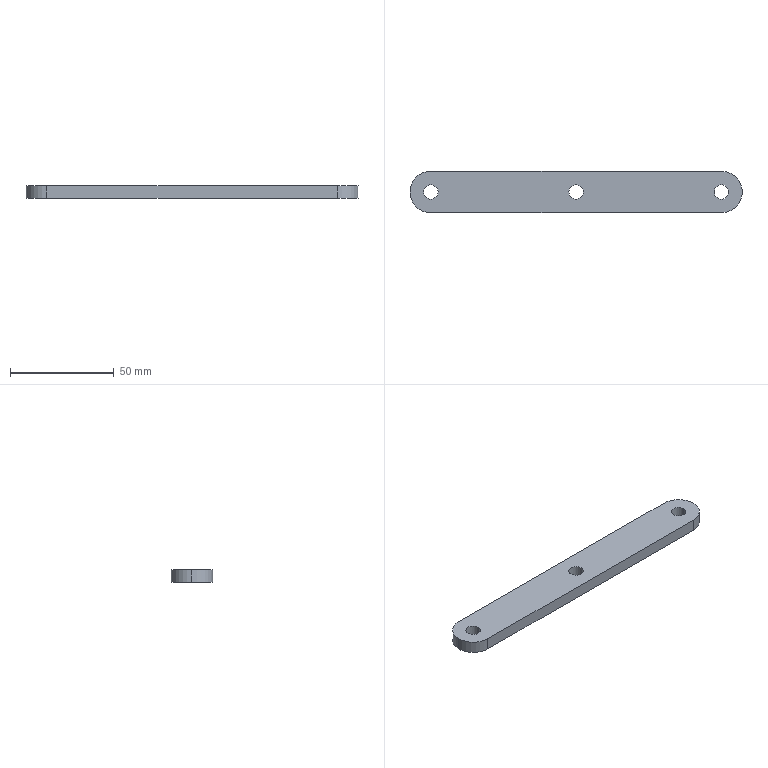Part | SolidWorks | features ICE 2, Extrusion 1 | 1 solid | 13 faces | box 160 x 20 x 6 mm | volume 17992 mm3 | cylinder 9 | plane 4 | commonest cylinder face diameters 7 x6 20 x3
STEP:
#1=CARTESIAN_POINT('',(66.5,0.,0.));
#2=VERTEX_POINT('',#1);
#3=CARTESIAN_POINT('',(73.5,0.,0.));
#4=VERTEX_POINT('',#3);
#5=CARTESIAN_POINT('',(70.,0.,0.));
#6=DIRECTION('',(0.,0.,1.));
#7=DIRECTION('',(1.,0.,0.));
#8=AXIS2_PLACEMENT_3D('',#5,#6,#7);
#9=CIRCLE('',#8,3.5);
#10=EDGE_CURVE('',#2,#4,#9,.T.);
#11=ORIENTED_EDGE('',*,*,#10,.F.);
#12=CARTESIAN_POINT('',(66.5,0.,6.));
#13=VERTEX_POINT('',#12);
#14=CARTESIAN_POINT('',(66.5,0.,-4.));
#15=DIRECTION('',(0.,0.,1.));
#16=VECTOR('',#15,1000.);
#17=LINE('',#14,#16);
#18=EDGE_CURVE('',#2,#13,#17,.T.);
#19=ORIENTED_EDGE('',*,*,#18,.T.);
#20=CARTESIAN_POINT('',(73.5,0.,6.));
#21=VERTEX_POINT('',#20);
#22=CARTESIAN_POINT('',(70.,0.,6.));
#23=DIRECTION('',(0.,0.,1.));
#24=DIRECTION('',(1.,0.,0.));
#25=AXIS2_PLACEMENT_3D('',#22,#23,#24);
#26=CIRCLE('',#25,3.5);
#27=EDGE_CURVE('',#13,#21,#26,.T.);
#28=ORIENTED_EDGE('',*,*,#27,.T.);
#29=CARTESIAN_POINT('',(73.5,0.,-4.));
#30=DIRECTION('',(0.,0.,1.));
#31=VECTOR('',#30,1000.);
#32=LINE('',#29,#31);
#33=EDGE_CURVE('',#4,#21,#32,.T.);
#34=ORIENTED_EDGE('',*,*,#33,.F.);
#35=EDGE_LOOP('',(#11,#19,#28,#34));
#36=FACE_OUTER_BOUND('',#35,.T.);
#37=CARTESIAN_POINT('',(70.,0.,-4.));
#38=DIRECTION('',(0.,0.,1.));
#39=DIRECTION('',(1.,0.,0.));
#40=AXIS2_PLACEMENT_3D('',#37,#38,#39);
#41=CYLINDRICAL_SURFACE('',#40,3.5);
#42=ADVANCED_FACE('',(#36),#41,.F.);
#43=CARTESIAN_POINT('',(136.5,0.,0.));
#44=VERTEX_POINT('',#43);
#45=CARTESIAN_POINT('',(143.5,0.,0.));
#46=VERTEX_POINT('',#45);
#47=CARTESIAN_POINT('',(140.,0.,0.));
#48=DIRECTION('',(0.,0.,1.));
#49=DIRECTION('',(1.,0.,0.));
#50=AXIS2_PLACEMENT_3D('',#47,#48,#49);
#51=CIRCLE('',#50,3.5);
#52=EDGE_CURVE('',#44,#46,#51,.T.);
#53=ORIENTED_EDGE('',*,*,#52,.F.);
#54=CARTESIAN_POINT('',(136.5,0.,6.));
#55=VERTEX_POINT('',#54);
#56=CARTESIAN_POINT('',(136.5,0.,-89.));
#57=DIRECTION('',(0.,0.,1.));
#58=VECTOR('',#57,1000.);
#59=LINE('',#56,#58);
#60=EDGE_CURVE('',#44,#55,#59,.T.);
#61=ORIENTED_EDGE('',*,*,#60,.T.);
#62=CARTESIAN_POINT('',(143.5,0.,6.));
#63=VERTEX_POINT('',#62);
#64=CARTESIAN_POINT('',(140.,0.,6.));
#65=DIRECTION('',(0.,0.,1.));
#66=DIRECTION('',(1.,0.,0.));
#67=AXIS2_PLACEMENT_3D('',#64,#65,#66);
#68=CIRCLE('',#67,3.5);
#69=EDGE_CURVE('',#55,#63,#68,.T.);
#70=ORIENTED_EDGE('',*,*,#69,.T.);
#71=CARTESIAN_POINT('',(143.5,0.,-89.));
#72=DIRECTION('',(0.,0.,1.));
#73=VECTOR('',#72,1000.);
#74=LINE('',#71,#73);
#75=EDGE_CURVE('',#46,#63,#74,.T.);
#76=ORIENTED_EDGE('',*,*,#75,.F.);
#77=EDGE_LOOP('',(#53,#61,#70,#76));
#78=FACE_OUTER_BOUND('',#77,.T.);
#79=CARTESIAN_POINT('',(140.,0.,-89.));
#80=DIRECTION('',(0.,0.,1.));
#81=DIRECTION('',(1.,0.,0.));
#82=AXIS2_PLACEMENT_3D('',#79,#80,#81);
#83=CYLINDRICAL_SURFACE('',#82,3.5);
#84=ADVANCED_FACE('',(#78),#83,.F.);
#85=CARTESIAN_POINT('',(-3.5,0.,0.));
#86=VERTEX_POINT('',#85);
#87=CARTESIAN_POINT('',(3.5,0.,0.));
#88=VERTEX_POINT('',#87);
#89=CARTESIAN_POINT('',(0.,0.,0.));
#90=DIRECTION('',(0.,0.,1.));
#91=DIRECTION('',(1.,0.,0.));
#92=AXIS2_PLACEMENT_3D('',#89,#90,#91);
#93=CIRCLE('',#92,3.5);
#94=EDGE_CURVE('',#86,#88,#93,.T.);
#95=ORIENTED_EDGE('',*,*,#94,.F.);
#96=CARTESIAN_POINT('',(-3.5,0.,6.));
#97=VERTEX_POINT('',#96);
#98=CARTESIAN_POINT('',(-3.5,0.,-89.));
#99=DIRECTION('',(0.,0.,1.));
#100=VECTOR('',#99,1000.);
#101=LINE('',#98,#100);
#102=EDGE_CURVE('',#86,#97,#101,.T.);
#103=ORIENTED_EDGE('',*,*,#102,.T.);
#104=CARTESIAN_POINT('',(3.5,0.,6.));
#105=VERTEX_POINT('',#104);
#106=CARTESIAN_POINT('',(0.,0.,6.));
#107=DIRECTION('',(0.,0.,1.));
#108=DIRECTION('',(1.,0.,0.));
#109=AXIS2_PLACEMENT_3D('',#106,#107,#108);
#110=CIRCLE('',#109,3.5);
#111=EDGE_CURVE('',#97,#105,#110,.T.);
#112=ORIENTED_EDGE('',*,*,#111,.T.);
#113=CARTESIAN_POINT('',(3.5,0.,-89.));
#114=DIRECTION('',(0.,0.,1.));
#115=VECTOR('',#114,1000.);
#116=LINE('',#113,#115);
#117=EDGE_CURVE('',#88,#105,#116,.T.);
#118=ORIENTED_EDGE('',*,*,#117,.F.);
#119=EDGE_LOOP('',(#95,#103,#112,#118));
#120=FACE_OUTER_BOUND('',#119,.T.);
#121=CARTESIAN_POINT('',(0.,0.,-89.));
#122=DIRECTION('',(0.,0.,1.));
#123=DIRECTION('',(1.,0.,0.));
#124=AXIS2_PLACEMENT_3D('',#121,#122,#123);
#125=CYLINDRICAL_SURFACE('',#124,3.5);
#126=ADVANCED_FACE('',(#120),#125,.F.);
#127=CARTESIAN_POINT('',(-10.,0.,6.));
#128=VERTEX_POINT('',#127);
#129=CARTESIAN_POINT('',(0.,-10.,6.));
#130=VERTEX_POINT('',#129);
#131=CARTESIAN_POINT('',(0.,0.,6.));
#132=DIRECTION('',(0.,0.,1.));
#133=DIRECTION('',(1.,0.,0.));
#134=AXIS2_PLACEMENT_3D('',#131,#132,#133);
#135=CIRCLE('',#134,10.);
#136=EDGE_CURVE('',#128,#130,#135,.T.);
#137=ORIENTED_EDGE('',*,*,#136,.F.);
#138=CARTESIAN_POINT('',(-10.,0.,0.));
#139=VERTEX_POINT('',#138);
#140=CARTESIAN_POINT('',(-10.,0.,6.));
#141=DIRECTION('',(0.,0.,-1.));
#142=VECTOR('',#141,1000.);
#143=LINE('',#140,#142);
#144=EDGE_CURVE('',#128,#139,#143,.T.);
#145=ORIENTED_EDGE('',*,*,#144,.T.);
#146=CARTESIAN_POINT('',(0.,-10.,0.));
#147=VERTEX_POINT('',#146);
#148=CARTESIAN_POINT('',(0.,0.,0.));
#149=DIRECTION('',(0.,0.,1.));
#150=DIRECTION('',(1.,0.,0.));
#151=AXIS2_PLACEMENT_3D('',#148,#149,#150);
#152=CIRCLE('',#151,10.);
#153=EDGE_CURVE('',#139,#147,#152,.T.);
#154=ORIENTED_EDGE('',*,*,#153,.T.);
#155=CARTESIAN_POINT('',(0.,-10.,6.));
#156=DIRECTION('',(0.,0.,-1.));
#157=VECTOR('',#156,1000.);
#158=LINE('',#155,#157);
#159=EDGE_CURVE('',#130,#147,#158,.T.);
#160=ORIENTED_EDGE('',*,*,#159,.F.);
#161=EDGE_LOOP('',(#137,#145,#154,#160));
#162=FACE_OUTER_BOUND('',#161,.T.);
#163=CARTESIAN_POINT('',(0.,0.,6.));
#164=DIRECTION('',(0.,0.,-1.));
#165=DIRECTION('',(-1.,0.,0.));
#166=AXIS2_PLACEMENT_3D('',#163,#164,#165);
#167=CYLINDRICAL_SURFACE('',#166,10.);
#168=ADVANCED_FACE('',(#162),#167,.T.);
#169=ORIENTED_EDGE('',*,*,#144,.F.);
#170=CARTESIAN_POINT('',(0.,10.,6.));
#171=VERTEX_POINT('',#170);
#172=CARTESIAN_POINT('',(0.,0.,6.));
#173=DIRECTION('',(0.,0.,1.));
#174=DIRECTION('',(1.,0.,0.));
#175=AXIS2_PLACEMENT_3D('',#172,#173,#174);
#176=CIRCLE('',#175,10.);
#177=EDGE_CURVE('',#171,#128,#176,.T.);
#178=ORIENTED_EDGE('',*,*,#177,.F.);
#179=CARTESIAN_POINT('',(0.,10.,0.));
#180=VERTEX_POINT('',#179);
#181=CARTESIAN_POINT('',(0.,10.,6.));
#182=DIRECTION('',(0.,0.,-1.));
#183=VECTOR('',#182,1000.);
#184=LINE('',#181,#183);
#185=EDGE_CURVE('',#171,#180,#184,.T.);
#186=ORIENTED_EDGE('',*,*,#185,.T.);
#187=CARTESIAN_POINT('',(0.,0.,0.));
#188=DIRECTION('',(0.,0.,1.));
#189=DIRECTION('',(1.,0.,0.));
#190=AXIS2_PLACEMENT_3D('',#187,#188,#189);
#191=CIRCLE('',#190,10.);
#192=EDGE_CURVE('',#180,#139,#191,.T.);
#193=ORIENTED_EDGE('',*,*,#192,.T.);
#194=EDGE_LOOP('',(#169,#178,#186,#193));
#195=FACE_OUTER_BOUND('',#194,.T.);
#196=CARTESIAN_POINT('',(0.,0.,6.));
#197=DIRECTION('',(0.,0.,-1.));
#198=DIRECTION('',(-1.,0.,0.));
#199=AXIS2_PLACEMENT_3D('',#196,#197,#198);
#200=CYLINDRICAL_SURFACE('',#199,10.);
#201=ADVANCED_FACE('',(#195),#200,.T.);
#202=CARTESIAN_POINT('',(140.,-10.,0.));
#203=VERTEX_POINT('',#202);
#204=CARTESIAN_POINT('',(0.,-10.,0.));
#205=DIRECTION('',(1.,0.,0.));
#206=VECTOR('',#205,1000.);
#207=LINE('',#204,#206);
#208=EDGE_CURVE('',#147,#203,#207,.T.);
#209=ORIENTED_EDGE('',*,*,#208,.T.);
#210=CARTESIAN_POINT('',(140.,-10.,6.));
#211=VERTEX_POINT('',#210);
#212=CARTESIAN_POINT('',(140.,-10.,6.));
#213=DIRECTION('',(0.,0.,-1.));
#214=VECTOR('',#213,1000.);
#215=LINE('',#212,#214);
#216=EDGE_CURVE('',#211,#203,#215,.T.);
#217=ORIENTED_EDGE('',*,*,#216,.F.);
#218=CARTESIAN_POINT('',(0.,-10.,6.));
#219=DIRECTION('',(1.,0.,0.));
#220=VECTOR('',#219,1000.);
#221=LINE('',#218,#220);
#222=EDGE_CURVE('',#130,#211,#221,.T.);
#223=ORIENTED_EDGE('',*,*,#222,.F.);
#224=ORIENTED_EDGE('',*,*,#159,.T.);
#225=EDGE_LOOP('',(#209,#217,#223,#224));
#226=FACE_OUTER_BOUND('',#225,.T.);
#227=CARTESIAN_POINT('',(0.,-10.,6.));
#228=DIRECTION('',(0.,1.,0.));
#229=DIRECTION('',(-1.,0.,0.));
#230=AXIS2_PLACEMENT_3D('',#227,#228,#229);
#231=PLANE('',#230);
#232=ADVANCED_FACE('',(#226),#231,.F.);
#233=CARTESIAN_POINT('',(140.,10.,0.));
#234=VERTEX_POINT('',#233);
#235=CARTESIAN_POINT('',(140.,0.,0.));
#236=DIRECTION('',(0.,0.,1.));
#237=DIRECTION('',(1.,0.,0.));
#238=AXIS2_PLACEMENT_3D('',#235,#236,#237);
#239=CIRCLE('',#238,10.);
#240=EDGE_CURVE('',#203,#234,#239,.T.);
#241=ORIENTED_EDGE('',*,*,#240,.T.);
#242=CARTESIAN_POINT('',(140.,10.,6.));
#243=VERTEX_POINT('',#242);
#244=CARTESIAN_POINT('',(140.,10.,6.));
#245=DIRECTION('',(0.,0.,-1.));
#246=VECTOR('',#245,1000.);
#247=LINE('',#244,#246);
#248=EDGE_CURVE('',#243,#234,#247,.T.);
#249=ORIENTED_EDGE('',*,*,#248,.F.);
#250=CARTESIAN_POINT('',(140.,0.,6.));
#251=DIRECTION('',(0.,0.,1.));
#252=DIRECTION('',(1.,0.,0.));
#253=AXIS2_PLACEMENT_3D('',#250,#251,#252);
#254=CIRCLE('',#253,10.);
#255=EDGE_CURVE('',#211,#243,#254,.T.);
#256=ORIENTED_EDGE('',*,*,#255,.F.);
#257=ORIENTED_EDGE('',*,*,#216,.T.);
#258=EDGE_LOOP('',(#241,#249,#256,#257));
#259=FACE_OUTER_BOUND('',#258,.T.);
#260=CARTESIAN_POINT('',(140.,0.,6.));
#261=DIRECTION('',(0.,0.,-1.));
#262=DIRECTION('',(-1.,0.,0.));
#263=AXIS2_PLACEMENT_3D('',#260,#261,#262);
#264=CYLINDRICAL_SURFACE('',#263,10.);
#265=ADVANCED_FACE('',(#259),#264,.T.);
#266=CARTESIAN_POINT('',(0.,10.,0.));
#267=DIRECTION('',(-1.,0.,0.));
#268=VECTOR('',#267,1000.);
#269=LINE('',#266,#268);
#270=EDGE_CURVE('',#234,#180,#269,.T.);
#271=ORIENTED_EDGE('',*,*,#270,.T.);
#272=ORIENTED_EDGE('',*,*,#185,.F.);
#273=CARTESIAN_POINT('',(0.,10.,6.));
#274=DIRECTION('',(-1.,0.,0.));
#275=VECTOR('',#274,1000.);
#276=LINE('',#273,#275);
#277=EDGE_CURVE('',#243,#171,#276,.T.);
#278=ORIENTED_EDGE('',*,*,#277,.F.);
#279=ORIENTED_EDGE('',*,*,#248,.T.);
#280=EDGE_LOOP('',(#271,#272,#278,#279));
#281=FACE_OUTER_BOUND('',#280,.T.);
#282=CARTESIAN_POINT('',(0.,10.,6.));
#283=DIRECTION('',(0.,-1.,0.));
#284=DIRECTION('',(1.,0.,0.));
#285=AXIS2_PLACEMENT_3D('',#282,#283,#284);
#286=PLANE('',#285);
#287=ADVANCED_FACE('',(#281),#286,.F.);
#288=CARTESIAN_POINT('',(70.,0.,6.));
#289=DIRECTION('',(0.,0.,1.));
#290=DIRECTION('',(1.,0.,0.));
#291=AXIS2_PLACEMENT_3D('',#288,#289,#290);
#292=CIRCLE('',#291,3.5);
#293=EDGE_CURVE('',#21,#13,#292,.T.);
#294=ORIENTED_EDGE('',*,*,#293,.F.);
#295=ORIENTED_EDGE('',*,*,#27,.F.);
#296=EDGE_LOOP('',(#294,#295));
#297=FACE_BOUND('',#296,.T.);
#298=CARTESIAN_POINT('',(140.,0.,6.));
#299=DIRECTION('',(0.,0.,1.));
#300=DIRECTION('',(1.,0.,0.));
#301=AXIS2_PLACEMENT_3D('',#298,#299,#300);
#302=CIRCLE('',#301,3.5);
#303=EDGE_CURVE('',#63,#55,#302,.T.);
#304=ORIENTED_EDGE('',*,*,#303,.F.);
#305=ORIENTED_EDGE('',*,*,#69,.F.);
#306=EDGE_LOOP('',(#304,#305));
#307=FACE_BOUND('',#306,.T.);
#308=CARTESIAN_POINT('',(0.,0.,6.));
#309=DIRECTION('',(0.,0.,1.));
#310=DIRECTION('',(1.,0.,0.));
#311=AXIS2_PLACEMENT_3D('',#308,#309,#310);
#312=CIRCLE('',#311,3.5);
#313=EDGE_CURVE('',#105,#97,#312,.T.);
#314=ORIENTED_EDGE('',*,*,#313,.F.);
#315=ORIENTED_EDGE('',*,*,#111,.F.);
#316=EDGE_LOOP('',(#314,#315));
#317=FACE_BOUND('',#316,.T.);
#318=ORIENTED_EDGE('',*,*,#177,.T.);
#319=ORIENTED_EDGE('',*,*,#136,.T.);
#320=ORIENTED_EDGE('',*,*,#222,.T.);
#321=ORIENTED_EDGE('',*,*,#255,.T.);
#322=ORIENTED_EDGE('',*,*,#277,.T.);
#323=EDGE_LOOP('',(#318,#319,#320,#321,#322));
#324=FACE_OUTER_BOUND('',#323,.T.);
#325=CARTESIAN_POINT('',(0.,0.,6.));
#326=DIRECTION('',(0.,0.,1.));
#327=DIRECTION('',(1.,0.,0.));
#328=AXIS2_PLACEMENT_3D('',#325,#326,#327);
#329=PLANE('',#328);
#330=ADVANCED_FACE('',(#297,#307,#317,#324),#329,.T.);
#331=CARTESIAN_POINT('',(70.,0.,0.));
#332=DIRECTION('',(0.,0.,1.));
#333=DIRECTION('',(1.,0.,0.));
#334=AXIS2_PLACEMENT_3D('',#331,#332,#333);
#335=CIRCLE('',#334,3.5);
#336=EDGE_CURVE('',#4,#2,#335,.T.);
#337=ORIENTED_EDGE('',*,*,#336,.T.);
#338=ORIENTED_EDGE('',*,*,#10,.T.);
#339=EDGE_LOOP('',(#337,#338));
#340=FACE_BOUND('',#339,.T.);
#341=CARTESIAN_POINT('',(140.,0.,0.));
#342=DIRECTION('',(0.,0.,1.));
#343=DIRECTION('',(1.,0.,0.));
#344=AXIS2_PLACEMENT_3D('',#341,#342,#343);
#345=CIRCLE('',#344,3.5);
#346=EDGE_CURVE('',#46,#44,#345,.T.);
#347=ORIENTED_EDGE('',*,*,#346,.T.);
#348=ORIENTED_EDGE('',*,*,#52,.T.);
#349=EDGE_LOOP('',(#347,#348));
#350=FACE_BOUND('',#349,.T.);
#351=CARTESIAN_POINT('',(0.,0.,0.));
#352=DIRECTION('',(0.,0.,1.));
#353=DIRECTION('',(1.,0.,0.));
#354=AXIS2_PLACEMENT_3D('',#351,#352,#353);
#355=CIRCLE('',#354,3.5);
#356=EDGE_CURVE('',#88,#86,#355,.T.);
#357=ORIENTED_EDGE('',*,*,#356,.T.);
#358=ORIENTED_EDGE('',*,*,#94,.T.);
#359=EDGE_LOOP('',(#357,#358));
#360=FACE_BOUND('',#359,.T.);
#361=ORIENTED_EDGE('',*,*,#192,.F.);
#362=ORIENTED_EDGE('',*,*,#270,.F.);
#363=ORIENTED_EDGE('',*,*,#240,.F.);
#364=ORIENTED_EDGE('',*,*,#208,.F.);
#365=ORIENTED_EDGE('',*,*,#153,.F.);
#366=EDGE_LOOP('',(#361,#362,#363,#364,#365));
#367=FACE_OUTER_BOUND('',#366,.T.);
#368=CARTESIAN_POINT('',(0.,0.,0.));
#369=DIRECTION('',(0.,0.,1.));
#370=DIRECTION('',(1.,0.,0.));
#371=AXIS2_PLACEMENT_3D('',#368,#369,#370);
#372=PLANE('',#371);
#373=ADVANCED_FACE('',(#340,#350,#360,#367),#372,.F.);
#374=ORIENTED_EDGE('',*,*,#102,.F.);
#375=ORIENTED_EDGE('',*,*,#356,.F.);
#376=ORIENTED_EDGE('',*,*,#117,.T.);
#377=ORIENTED_EDGE('',*,*,#313,.T.);
#378=EDGE_LOOP('',(#374,#375,#376,#377));
#379=FACE_OUTER_BOUND('',#378,.T.);
#380=CARTESIAN_POINT('',(0.,0.,-89.));
#381=DIRECTION('',(0.,0.,1.));
#382=DIRECTION('',(1.,0.,0.));
#383=AXIS2_PLACEMENT_3D('',#380,#381,#382);
#384=CYLINDRICAL_SURFACE('',#383,3.5);
#385=ADVANCED_FACE('',(#379),#384,.F.);
#386=ORIENTED_EDGE('',*,*,#60,.F.);
#387=ORIENTED_EDGE('',*,*,#346,.F.);
#388=ORIENTED_EDGE('',*,*,#75,.T.);
#389=ORIENTED_EDGE('',*,*,#303,.T.);
#390=EDGE_LOOP('',(#386,#387,#388,#389));
#391=FACE_OUTER_BOUND('',#390,.T.);
#392=CARTESIAN_POINT('',(140.,0.,-89.));
#393=DIRECTION('',(0.,0.,1.));
#394=DIRECTION('',(1.,0.,0.));
#395=AXIS2_PLACEMENT_3D('',#392,#393,#394);
#396=CYLINDRICAL_SURFACE('',#395,3.5);
#397=ADVANCED_FACE('',(#391),#396,.F.);
#398=ORIENTED_EDGE('',*,*,#18,.F.);
#399=ORIENTED_EDGE('',*,*,#336,.F.);
#400=ORIENTED_EDGE('',*,*,#33,.T.);
#401=ORIENTED_EDGE('',*,*,#293,.T.);
#402=EDGE_LOOP('',(#398,#399,#400,#401));
#403=FACE_OUTER_BOUND('',#402,.T.);
#404=CARTESIAN_POINT('',(70.,0.,-4.));
#405=DIRECTION('',(0.,0.,1.));
#406=DIRECTION('',(1.,0.,0.));
#407=AXIS2_PLACEMENT_3D('',#404,#405,#406);
#408=CYLINDRICAL_SURFACE('',#407,3.5);
#409=ADVANCED_FACE('',(#403),#408,.F.);
#410=CLOSED_SHELL('',(#42,#84,#126,#168,#201,#232,#265,#287,#330,#373,#385,#397,#409));
#411=MANIFOLD_SOLID_BREP('',#410);
#412=CARTESIAN_POINT('',(0.,0.,0.));
#413=DIRECTION('',(0.,0.,1.));
#414=DIRECTION('',(1.,0.,0.));
#415=AXIS2_PLACEMENT_3D('',#412,#413,#414);
#416=(LENGTH_UNIT()NAMED_UNIT(*)SI_UNIT(.MILLI.,.METRE.));
#417=UNCERTAINTY_MEASURE_WITH_UNIT(LENGTH_MEASURE(0.00001),#416,'','');
#418=(NAMED_UNIT(*)PLANE_ANGLE_UNIT()SI_UNIT($,.RADIAN.));
#419=(NAMED_UNIT(*)SI_UNIT($,.STERADIAN.)SOLID_ANGLE_UNIT());
#420=(GEOMETRIC_REPRESENTATION_CONTEXT(3)GLOBAL_UNCERTAINTY_ASSIGNED_CONTEXT((#417))GLOBAL_UNIT_ASSIGNED_CONTEXT((#416,#418,#419))REPRESENTATION_CONTEXT('',''));
#421=ADVANCED_BREP_SHAPE_REPRESENTATION('',(#411,#415),#420);